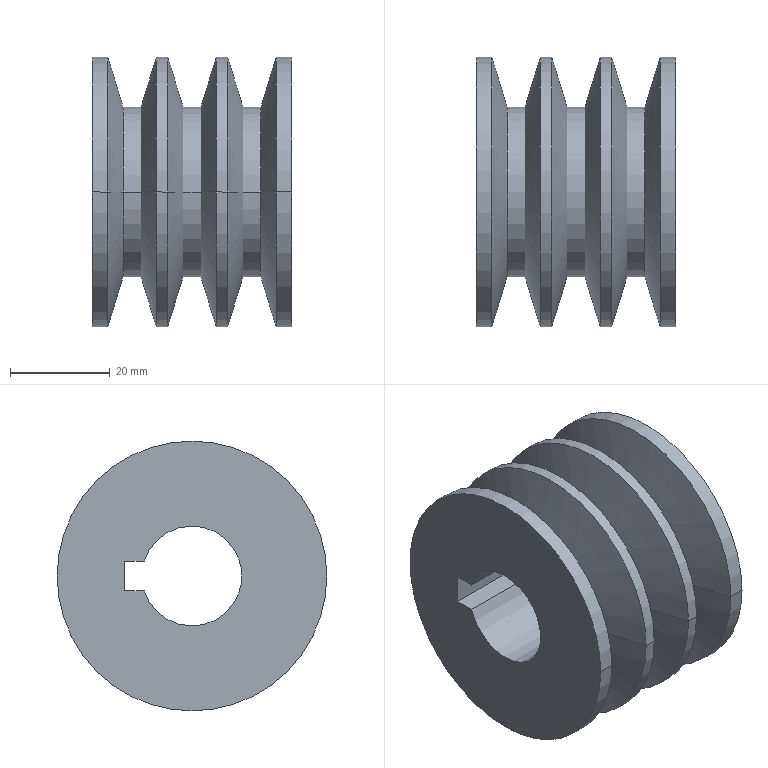Part | STEP file | Constant-speed small pulley | 1 solid | 32 faces | box 40 x 54 x 54 mm | volume 49564 mm3 | cylinder 15 | cone 12 | plane 5 | commonest cylinder face diameters 54 x8 34 x6 20 x1
STEP:
#1=CARTESIAN_POINT('',(-3.139,27.,0.));
#2=VERTEX_POINT('',#1);
#3=CARTESIAN_POINT('',(-3.139,-27.,0.));
#4=VERTEX_POINT('',#3);
#5=CARTESIAN_POINT('',(-3.139,0.,0.));
#6=DIRECTION('',(1.,0.,0.));
#7=DIRECTION('',(0.,1.,0.));
#8=AXIS2_PLACEMENT_3D('',#5,#6,#7);
#9=CIRCLE('',#8,27.);
#10=EDGE_CURVE('',#2,#4,#9,.T.);
#11=ORIENTED_EDGE('',*,*,#10,.T.);
#12=CARTESIAN_POINT('',(0.,-27.,0.));
#13=VERTEX_POINT('',#12);
#14=CARTESIAN_POINT('',(22.861,-27.,0.));
#15=DIRECTION('',(1.,0.,0.));
#16=VECTOR('',#15,1000.);
#17=LINE('',#14,#16);
#18=EDGE_CURVE('',#4,#13,#17,.T.);
#19=ORIENTED_EDGE('',*,*,#18,.T.);
#20=CARTESIAN_POINT('',(0.,27.,0.));
#21=VERTEX_POINT('',#20);
#22=CARTESIAN_POINT('',(0.,0.,0.));
#23=DIRECTION('',(1.,0.,0.));
#24=DIRECTION('',(0.,1.,0.));
#25=AXIS2_PLACEMENT_3D('',#22,#23,#24);
#26=CIRCLE('',#25,27.);
#27=EDGE_CURVE('',#21,#13,#26,.T.);
#28=ORIENTED_EDGE('',*,*,#27,.F.);
#29=CARTESIAN_POINT('',(22.861,27.,0.));
#30=DIRECTION('',(1.,0.,0.));
#31=VECTOR('',#30,1000.);
#32=LINE('',#29,#31);
#33=EDGE_CURVE('',#2,#21,#32,.T.);
#34=ORIENTED_EDGE('',*,*,#33,.F.);
#35=EDGE_LOOP('',(#11,#19,#28,#34));
#36=FACE_OUTER_BOUND('',#35,.T.);
#37=CARTESIAN_POINT('',(22.861,0.,0.));
#38=DIRECTION('',(1.,0.,0.));
#39=DIRECTION('',(0.,1.,0.));
#40=AXIS2_PLACEMENT_3D('',#37,#38,#39);
#41=CYLINDRICAL_SURFACE('',#40,27.);
#42=ADVANCED_FACE('',(#36),#41,.T.);
#43=CARTESIAN_POINT('',(3.057,17.,0.));
#44=VERTEX_POINT('',#43);
#45=CARTESIAN_POINT('',(3.057,-17.,0.));
#46=VERTEX_POINT('',#45);
#47=CARTESIAN_POINT('',(3.057,0.,0.));
#48=DIRECTION('',(1.,0.,0.));
#49=DIRECTION('',(0.,1.,0.));
#50=AXIS2_PLACEMENT_3D('',#47,#48,#49);
#51=CIRCLE('',#50,17.);
#52=EDGE_CURVE('',#44,#46,#51,.T.);
#53=ORIENTED_EDGE('',*,*,#52,.F.);
#54=CARTESIAN_POINT('',(3.057,17.,0.));
#55=DIRECTION('',(-0.2924,0.9563,0.));
#56=VECTOR('',#55,1000.);
#57=LINE('',#54,#56);
#58=EDGE_CURVE('',#44,#21,#57,.T.);
#59=ORIENTED_EDGE('',*,*,#58,.T.);
#60=ORIENTED_EDGE('',*,*,#27,.T.);
#61=CARTESIAN_POINT('',(3.057,-17.,0.));
#62=DIRECTION('',(-0.2924,-0.9563,0.));
#63=VECTOR('',#62,1000.);
#64=LINE('',#61,#63);
#65=EDGE_CURVE('',#46,#13,#64,.T.);
#66=ORIENTED_EDGE('',*,*,#65,.F.);
#67=EDGE_LOOP('',(#53,#59,#60,#66));
#68=FACE_OUTER_BOUND('',#67,.T.);
#69=CARTESIAN_POINT('',(3.057,0.,0.));
#70=DIRECTION('',(-1.,0.,0.));
#71=DIRECTION('',(0.,-1.,0.));
#72=AXIS2_PLACEMENT_3D('',#69,#70,#71);
#73=CONICAL_SURFACE('',#72,17.,1.274);
#74=ADVANCED_FACE('',(#68),#73,.T.);
#75=ORIENTED_EDGE('',*,*,#52,.T.);
#76=CARTESIAN_POINT('',(6.666,-17.,0.));
#77=VERTEX_POINT('',#76);
#78=CARTESIAN_POINT('',(22.861,-17.,0.));
#79=DIRECTION('',(1.,0.,0.));
#80=VECTOR('',#79,1000.);
#81=LINE('',#78,#80);
#82=EDGE_CURVE('',#46,#77,#81,.T.);
#83=ORIENTED_EDGE('',*,*,#82,.T.);
#84=CARTESIAN_POINT('',(6.666,17.,0.));
#85=VERTEX_POINT('',#84);
#86=CARTESIAN_POINT('',(6.666,0.,0.));
#87=DIRECTION('',(1.,0.,0.));
#88=DIRECTION('',(0.,1.,0.));
#89=AXIS2_PLACEMENT_3D('',#86,#87,#88);
#90=CIRCLE('',#89,17.);
#91=EDGE_CURVE('',#85,#77,#90,.T.);
#92=ORIENTED_EDGE('',*,*,#91,.F.);
#93=CARTESIAN_POINT('',(22.861,17.,0.));
#94=DIRECTION('',(1.,0.,0.));
#95=VECTOR('',#94,1000.);
#96=LINE('',#93,#95);
#97=EDGE_CURVE('',#44,#85,#96,.T.);
#98=ORIENTED_EDGE('',*,*,#97,.F.);
#99=EDGE_LOOP('',(#75,#83,#92,#98));
#100=FACE_OUTER_BOUND('',#99,.T.);
#101=CARTESIAN_POINT('',(22.861,0.,0.));
#102=DIRECTION('',(1.,0.,0.));
#103=DIRECTION('',(0.,1.,0.));
#104=AXIS2_PLACEMENT_3D('',#101,#102,#103);
#105=CYLINDRICAL_SURFACE('',#104,17.);
#106=ADVANCED_FACE('',(#100),#105,.T.);
#107=ORIENTED_EDGE('',*,*,#91,.T.);
#108=CARTESIAN_POINT('',(9.723,-27.,0.));
#109=VERTEX_POINT('',#108);
#110=CARTESIAN_POINT('',(9.723,-27.,0.));
#111=DIRECTION('',(0.2924,-0.9563,0.));
#112=VECTOR('',#111,1000.);
#113=LINE('',#110,#112);
#114=EDGE_CURVE('',#77,#109,#113,.T.);
#115=ORIENTED_EDGE('',*,*,#114,.T.);
#116=CARTESIAN_POINT('',(9.723,27.,0.));
#117=VERTEX_POINT('',#116);
#118=CARTESIAN_POINT('',(9.723,0.,0.));
#119=DIRECTION('',(1.,0.,0.));
#120=DIRECTION('',(0.,1.,0.));
#121=AXIS2_PLACEMENT_3D('',#118,#119,#120);
#122=CIRCLE('',#121,27.);
#123=EDGE_CURVE('',#117,#109,#122,.T.);
#124=ORIENTED_EDGE('',*,*,#123,.F.);
#125=CARTESIAN_POINT('',(9.723,27.,0.));
#126=DIRECTION('',(0.2924,0.9563,0.));
#127=VECTOR('',#126,1000.);
#128=LINE('',#125,#127);
#129=EDGE_CURVE('',#85,#117,#128,.T.);
#130=ORIENTED_EDGE('',*,*,#129,.F.);
#131=EDGE_LOOP('',(#107,#115,#124,#130));
#132=FACE_OUTER_BOUND('',#131,.T.);
#133=CARTESIAN_POINT('',(9.723,0.,0.));
#134=DIRECTION('',(1.,0.,0.));
#135=DIRECTION('',(0.,1.,0.));
#136=AXIS2_PLACEMENT_3D('',#133,#134,#135);
#137=CONICAL_SURFACE('',#136,27.,1.274);
#138=ADVANCED_FACE('',(#132),#137,.T.);
#139=ORIENTED_EDGE('',*,*,#123,.T.);
#140=CARTESIAN_POINT('',(12.,-27.,0.));
#141=VERTEX_POINT('',#140);
#142=CARTESIAN_POINT('',(22.861,-27.,0.));
#143=DIRECTION('',(1.,0.,0.));
#144=VECTOR('',#143,1000.);
#145=LINE('',#142,#144);
#146=EDGE_CURVE('',#109,#141,#145,.T.);
#147=ORIENTED_EDGE('',*,*,#146,.T.);
#148=CARTESIAN_POINT('',(12.,27.,0.));
#149=VERTEX_POINT('',#148);
#150=CARTESIAN_POINT('',(12.,0.,0.));
#151=DIRECTION('',(1.,0.,0.));
#152=DIRECTION('',(0.,1.,0.));
#153=AXIS2_PLACEMENT_3D('',#150,#151,#152);
#154=CIRCLE('',#153,27.);
#155=EDGE_CURVE('',#149,#141,#154,.T.);
#156=ORIENTED_EDGE('',*,*,#155,.F.);
#157=CARTESIAN_POINT('',(22.861,27.,0.));
#158=DIRECTION('',(1.,0.,0.));
#159=VECTOR('',#158,1000.);
#160=LINE('',#157,#159);
#161=EDGE_CURVE('',#117,#149,#160,.T.);
#162=ORIENTED_EDGE('',*,*,#161,.F.);
#163=EDGE_LOOP('',(#139,#147,#156,#162));
#164=FACE_OUTER_BOUND('',#163,.T.);
#165=CARTESIAN_POINT('',(22.861,0.,0.));
#166=DIRECTION('',(1.,0.,0.));
#167=DIRECTION('',(0.,1.,0.));
#168=AXIS2_PLACEMENT_3D('',#165,#166,#167);
#169=CYLINDRICAL_SURFACE('',#168,27.);
#170=ADVANCED_FACE('',(#164),#169,.T.);
#171=CARTESIAN_POINT('',(15.057,17.,0.));
#172=VERTEX_POINT('',#171);
#173=CARTESIAN_POINT('',(15.057,-17.,0.));
#174=VERTEX_POINT('',#173);
#175=CARTESIAN_POINT('',(15.057,0.,0.));
#176=DIRECTION('',(1.,0.,0.));
#177=DIRECTION('',(0.,1.,0.));
#178=AXIS2_PLACEMENT_3D('',#175,#176,#177);
#179=CIRCLE('',#178,17.);
#180=EDGE_CURVE('',#172,#174,#179,.T.);
#181=ORIENTED_EDGE('',*,*,#180,.F.);
#182=CARTESIAN_POINT('',(15.057,17.,0.));
#183=DIRECTION('',(-0.2924,0.9563,0.));
#184=VECTOR('',#183,1000.);
#185=LINE('',#182,#184);
#186=EDGE_CURVE('',#172,#149,#185,.T.);
#187=ORIENTED_EDGE('',*,*,#186,.T.);
#188=ORIENTED_EDGE('',*,*,#155,.T.);
#189=CARTESIAN_POINT('',(15.057,-17.,0.));
#190=DIRECTION('',(-0.2924,-0.9563,0.));
#191=VECTOR('',#190,1000.);
#192=LINE('',#189,#191);
#193=EDGE_CURVE('',#174,#141,#192,.T.);
#194=ORIENTED_EDGE('',*,*,#193,.F.);
#195=EDGE_LOOP('',(#181,#187,#188,#194));
#196=FACE_OUTER_BOUND('',#195,.T.);
#197=CARTESIAN_POINT('',(15.057,0.,0.));
#198=DIRECTION('',(-1.,0.,0.));
#199=DIRECTION('',(0.,-1.,0.));
#200=AXIS2_PLACEMENT_3D('',#197,#198,#199);
#201=CONICAL_SURFACE('',#200,17.,1.274);
#202=ADVANCED_FACE('',(#196),#201,.T.);
#203=ORIENTED_EDGE('',*,*,#180,.T.);
#204=CARTESIAN_POINT('',(18.666,-17.,0.));
#205=VERTEX_POINT('',#204);
#206=CARTESIAN_POINT('',(22.861,-17.,0.));
#207=DIRECTION('',(1.,0.,0.));
#208=VECTOR('',#207,1000.);
#209=LINE('',#206,#208);
#210=EDGE_CURVE('',#174,#205,#209,.T.);
#211=ORIENTED_EDGE('',*,*,#210,.T.);
#212=CARTESIAN_POINT('',(18.666,17.,0.));
#213=VERTEX_POINT('',#212);
#214=CARTESIAN_POINT('',(18.666,0.,0.));
#215=DIRECTION('',(1.,0.,0.));
#216=DIRECTION('',(0.,1.,0.));
#217=AXIS2_PLACEMENT_3D('',#214,#215,#216);
#218=CIRCLE('',#217,17.);
#219=EDGE_CURVE('',#213,#205,#218,.T.);
#220=ORIENTED_EDGE('',*,*,#219,.F.);
#221=CARTESIAN_POINT('',(22.861,17.,0.));
#222=DIRECTION('',(1.,0.,0.));
#223=VECTOR('',#222,1000.);
#224=LINE('',#221,#223);
#225=EDGE_CURVE('',#172,#213,#224,.T.);
#226=ORIENTED_EDGE('',*,*,#225,.F.);
#227=EDGE_LOOP('',(#203,#211,#220,#226));
#228=FACE_OUTER_BOUND('',#227,.T.);
#229=CARTESIAN_POINT('',(22.861,0.,0.));
#230=DIRECTION('',(1.,0.,0.));
#231=DIRECTION('',(0.,1.,0.));
#232=AXIS2_PLACEMENT_3D('',#229,#230,#231);
#233=CYLINDRICAL_SURFACE('',#232,17.);
#234=ADVANCED_FACE('',(#228),#233,.T.);
#235=ORIENTED_EDGE('',*,*,#219,.T.);
#236=CARTESIAN_POINT('',(21.723,-27.,0.));
#237=VERTEX_POINT('',#236);
#238=CARTESIAN_POINT('',(21.723,-27.,0.));
#239=DIRECTION('',(0.2924,-0.9563,0.));
#240=VECTOR('',#239,1000.);
#241=LINE('',#238,#240);
#242=EDGE_CURVE('',#205,#237,#241,.T.);
#243=ORIENTED_EDGE('',*,*,#242,.T.);
#244=CARTESIAN_POINT('',(21.723,27.,0.));
#245=VERTEX_POINT('',#244);
#246=CARTESIAN_POINT('',(21.723,0.,0.));
#247=DIRECTION('',(1.,0.,0.));
#248=DIRECTION('',(0.,1.,0.));
#249=AXIS2_PLACEMENT_3D('',#246,#247,#248);
#250=CIRCLE('',#249,27.);
#251=EDGE_CURVE('',#245,#237,#250,.T.);
#252=ORIENTED_EDGE('',*,*,#251,.F.);
#253=CARTESIAN_POINT('',(21.723,27.,0.));
#254=DIRECTION('',(0.2924,0.9563,0.));
#255=VECTOR('',#254,1000.);
#256=LINE('',#253,#255);
#257=EDGE_CURVE('',#213,#245,#256,.T.);
#258=ORIENTED_EDGE('',*,*,#257,.F.);
#259=EDGE_LOOP('',(#235,#243,#252,#258));
#260=FACE_OUTER_BOUND('',#259,.T.);
#261=CARTESIAN_POINT('',(21.723,0.,0.));
#262=DIRECTION('',(1.,0.,0.));
#263=DIRECTION('',(0.,1.,0.));
#264=AXIS2_PLACEMENT_3D('',#261,#262,#263);
#265=CONICAL_SURFACE('',#264,27.,1.274);
#266=ADVANCED_FACE('',(#260),#265,.T.);
#267=ORIENTED_EDGE('',*,*,#251,.T.);
#268=CARTESIAN_POINT('',(24.,-27.,0.));
#269=VERTEX_POINT('',#268);
#270=CARTESIAN_POINT('',(22.861,-27.,0.));
#271=DIRECTION('',(1.,0.,0.));
#272=VECTOR('',#271,1000.);
#273=LINE('',#270,#272);
#274=EDGE_CURVE('',#237,#269,#273,.T.);
#275=ORIENTED_EDGE('',*,*,#274,.T.);
#276=CARTESIAN_POINT('',(24.,27.,0.));
#277=VERTEX_POINT('',#276);
#278=CARTESIAN_POINT('',(24.,0.,0.));
#279=DIRECTION('',(1.,0.,0.));
#280=DIRECTION('',(0.,1.,0.));
#281=AXIS2_PLACEMENT_3D('',#278,#279,#280);
#282=CIRCLE('',#281,27.);
#283=EDGE_CURVE('',#277,#269,#282,.T.);
#284=ORIENTED_EDGE('',*,*,#283,.F.);
#285=CARTESIAN_POINT('',(22.861,27.,0.));
#286=DIRECTION('',(1.,0.,0.));
#287=VECTOR('',#286,1000.);
#288=LINE('',#285,#287);
#289=EDGE_CURVE('',#245,#277,#288,.T.);
#290=ORIENTED_EDGE('',*,*,#289,.F.);
#291=EDGE_LOOP('',(#267,#275,#284,#290));
#292=FACE_OUTER_BOUND('',#291,.T.);
#293=CARTESIAN_POINT('',(22.861,0.,0.));
#294=DIRECTION('',(1.,0.,0.));
#295=DIRECTION('',(0.,1.,0.));
#296=AXIS2_PLACEMENT_3D('',#293,#294,#295);
#297=CYLINDRICAL_SURFACE('',#296,27.);
#298=ADVANCED_FACE('',(#292),#297,.T.);
#299=CARTESIAN_POINT('',(27.057,17.,0.));
#300=VERTEX_POINT('',#299);
#301=CARTESIAN_POINT('',(27.057,-17.,0.));
#302=VERTEX_POINT('',#301);
#303=CARTESIAN_POINT('',(27.057,0.,0.));
#304=DIRECTION('',(1.,0.,0.));
#305=DIRECTION('',(0.,1.,0.));
#306=AXIS2_PLACEMENT_3D('',#303,#304,#305);
#307=CIRCLE('',#306,17.);
#308=EDGE_CURVE('',#300,#302,#307,.T.);
#309=ORIENTED_EDGE('',*,*,#308,.F.);
#310=CARTESIAN_POINT('',(27.057,17.,0.));
#311=DIRECTION('',(-0.2924,0.9563,0.));
#312=VECTOR('',#311,1000.);
#313=LINE('',#310,#312);
#314=EDGE_CURVE('',#300,#277,#313,.T.);
#315=ORIENTED_EDGE('',*,*,#314,.T.);
#316=ORIENTED_EDGE('',*,*,#283,.T.);
#317=CARTESIAN_POINT('',(27.057,-17.,0.));
#318=DIRECTION('',(-0.2924,-0.9563,0.));
#319=VECTOR('',#318,1000.);
#320=LINE('',#317,#319);
#321=EDGE_CURVE('',#302,#269,#320,.T.);
#322=ORIENTED_EDGE('',*,*,#321,.F.);
#323=EDGE_LOOP('',(#309,#315,#316,#322));
#324=FACE_OUTER_BOUND('',#323,.T.);
#325=CARTESIAN_POINT('',(27.057,0.,0.));
#326=DIRECTION('',(-1.,0.,0.));
#327=DIRECTION('',(0.,-1.,0.));
#328=AXIS2_PLACEMENT_3D('',#325,#326,#327);
#329=CONICAL_SURFACE('',#328,17.,1.274);
#330=ADVANCED_FACE('',(#324),#329,.T.);
#331=ORIENTED_EDGE('',*,*,#308,.T.);
#332=CARTESIAN_POINT('',(30.666,-17.,0.));
#333=VERTEX_POINT('',#332);
#334=CARTESIAN_POINT('',(22.861,-17.,0.));
#335=DIRECTION('',(1.,0.,0.));
#336=VECTOR('',#335,1000.);
#337=LINE('',#334,#336);
#338=EDGE_CURVE('',#302,#333,#337,.T.);
#339=ORIENTED_EDGE('',*,*,#338,.T.);
#340=CARTESIAN_POINT('',(30.666,17.,0.));
#341=VERTEX_POINT('',#340);
#342=CARTESIAN_POINT('',(30.666,0.,0.));
#343=DIRECTION('',(1.,0.,0.));
#344=DIRECTION('',(0.,1.,0.));
#345=AXIS2_PLACEMENT_3D('',#342,#343,#344);
#346=CIRCLE('',#345,17.);
#347=EDGE_CURVE('',#341,#333,#346,.T.);
#348=ORIENTED_EDGE('',*,*,#347,.F.);
#349=CARTESIAN_POINT('',(22.861,17.,0.));
#350=DIRECTION('',(1.,0.,0.));
#351=VECTOR('',#350,1000.);
#352=LINE('',#349,#351);
#353=EDGE_CURVE('',#300,#341,#352,.T.);
#354=ORIENTED_EDGE('',*,*,#353,.F.);
#355=EDGE_LOOP('',(#331,#339,#348,#354));
#356=FACE_OUTER_BOUND('',#355,.T.);
#357=CARTESIAN_POINT('',(22.861,0.,0.));
#358=DIRECTION('',(1.,0.,0.));
#359=DIRECTION('',(0.,1.,0.));
#360=AXIS2_PLACEMENT_3D('',#357,#358,#359);
#361=CYLINDRICAL_SURFACE('',#360,17.);
#362=ADVANCED_FACE('',(#356),#361,.T.);
#363=ORIENTED_EDGE('',*,*,#347,.T.);
#364=CARTESIAN_POINT('',(33.723,-27.,0.));
#365=VERTEX_POINT('',#364);
#366=CARTESIAN_POINT('',(33.723,-27.,0.));
#367=DIRECTION('',(0.2924,-0.9563,0.));
#368=VECTOR('',#367,1000.);
#369=LINE('',#366,#368);
#370=EDGE_CURVE('',#333,#365,#369,.T.);
#371=ORIENTED_EDGE('',*,*,#370,.T.);
#372=CARTESIAN_POINT('',(33.723,27.,0.));
#373=VERTEX_POINT('',#372);
#374=CARTESIAN_POINT('',(33.723,0.,0.));
#375=DIRECTION('',(1.,0.,0.));
#376=DIRECTION('',(0.,1.,0.));
#377=AXIS2_PLACEMENT_3D('',#374,#375,#376);
#378=CIRCLE('',#377,27.);
#379=EDGE_CURVE('',#373,#365,#378,.T.);
#380=ORIENTED_EDGE('',*,*,#379,.F.);
#381=CARTESIAN_POINT('',(33.723,27.,0.));
#382=DIRECTION('',(0.2924,0.9563,0.));
#383=VECTOR('',#382,1000.);
#384=LINE('',#381,#383);
#385=EDGE_CURVE('',#341,#373,#384,.T.);
#386=ORIENTED_EDGE('',*,*,#385,.F.);
#387=EDGE_LOOP('',(#363,#371,#380,#386));
#388=FACE_OUTER_BOUND('',#387,.T.);
#389=CARTESIAN_POINT('',(33.723,0.,0.));
#390=DIRECTION('',(1.,0.,0.));
#391=DIRECTION('',(0.,1.,0.));
#392=AXIS2_PLACEMENT_3D('',#389,#390,#391);
#393=CONICAL_SURFACE('',#392,27.,1.274);
#394=ADVANCED_FACE('',(#388),#393,.T.);
#395=ORIENTED_EDGE('',*,*,#379,.T.);
#396=CARTESIAN_POINT('',(36.861,-27.,0.));
#397=VERTEX_POINT('',#396);
#398=CARTESIAN_POINT('',(22.861,-27.,0.));
#399=DIRECTION('',(1.,0.,0.));
#400=VECTOR('',#399,1000.);
#401=LINE('',#398,#400);
#402=EDGE_CURVE('',#365,#397,#401,.T.);
#403=ORIENTED_EDGE('',*,*,#402,.T.);
#404=CARTESIAN_POINT('',(36.861,27.,0.));
#405=VERTEX_POINT('',#404);
#406=CARTESIAN_POINT('',(36.861,0.,0.));
#407=DIRECTION('',(1.,0.,0.));
#408=DIRECTION('',(0.,1.,0.));
#409=AXIS2_PLACEMENT_3D('',#406,#407,#408);
#410=CIRCLE('',#409,27.);
#411=EDGE_CURVE('',#405,#397,#410,.T.);
#412=ORIENTED_EDGE('',*,*,#411,.F.);
#413=CARTESIAN_POINT('',(22.861,27.,0.));
#414=DIRECTION('',(1.,0.,0.));
#415=VECTOR('',#414,1000.);
#416=LINE('',#413,#415);
#417=EDGE_CURVE('',#373,#405,#416,.T.);
#418=ORIENTED_EDGE('',*,*,#417,.F.);
#419=EDGE_LOOP('',(#395,#403,#412,#418));
#420=FACE_OUTER_BOUND('',#419,.T.);
#421=CARTESIAN_POINT('',(22.861,0.,0.));
#422=DIRECTION('',(1.,0.,0.));
#423=DIRECTION('',(0.,1.,0.));
#424=AXIS2_PLACEMENT_3D('',#421,#422,#423);
#425=CYLINDRICAL_SURFACE('',#424,27.);
#426=ADVANCED_FACE('',(#420),#425,.T.);
#427=CARTESIAN_POINT('',(-3.139,13.5,-3.));
#428=VERTEX_POINT('',#427);
#429=CARTESIAN_POINT('',(-3.139,9.539,-3.));
#430=VERTEX_POINT('',#429);
#431=CARTESIAN_POINT('',(-3.139,27.,-3.));
#432=DIRECTION('',(0.,-1.,0.));
#433=VECTOR('',#432,1000.);
#434=LINE('',#431,#433);
#435=EDGE_CURVE('',#428,#430,#434,.T.);
#436=ORIENTED_EDGE('',*,*,#435,.F.);
#437=CARTESIAN_POINT('',(-3.139,13.5,3.));
#438=VERTEX_POINT('',#437);
#439=CARTESIAN_POINT('',(-3.139,13.5,0.));
#440=DIRECTION('',(0.,0.,-1.));
#441=VECTOR('',#440,1000.);
#442=LINE('',#439,#441);
#443=EDGE_CURVE('',#438,#428,#442,.T.);
#444=ORIENTED_EDGE('',*,*,#443,.F.);
#445=CARTESIAN_POINT('',(-3.139,9.539,3.));
#446=VERTEX_POINT('',#445);
#447=CARTESIAN_POINT('',(-3.139,27.,3.));
#448=DIRECTION('',(0.,1.,0.));
#449=VECTOR('',#448,1000.);
#450=LINE('',#447,#449);
#451=EDGE_CURVE('',#446,#438,#450,.T.);
#452=ORIENTED_EDGE('',*,*,#451,.F.);
#453=CARTESIAN_POINT('',(-3.139,0.,0.));
#454=DIRECTION('',(-1.,0.,0.));
#455=DIRECTION('',(0.,-1.,0.));
#456=AXIS2_PLACEMENT_3D('',#453,#454,#455);
#457=CIRCLE('',#456,10.);
#458=EDGE_CURVE('',#430,#446,#457,.T.);
#459=ORIENTED_EDGE('',*,*,#458,.F.);
#460=EDGE_LOOP('',(#436,#444,#452,#459));
#461=FACE_BOUND('',#460,.T.);
#462=ORIENTED_EDGE('',*,*,#10,.F.);
#463=CARTESIAN_POINT('',(-3.139,0.,0.));
#464=DIRECTION('',(1.,0.,0.));
#465=DIRECTION('',(0.,1.,0.));
#466=AXIS2_PLACEMENT_3D('',#463,#464,#465);
#467=CIRCLE('',#466,27.);
#468=EDGE_CURVE('',#4,#2,#467,.T.);
#469=ORIENTED_EDGE('',*,*,#468,.F.);
#470=EDGE_LOOP('',(#462,#469));
#471=FACE_OUTER_BOUND('',#470,.T.);
#472=CARTESIAN_POINT('',(-3.139,27.,0.));
#473=DIRECTION('',(-1.,0.,0.));
#474=DIRECTION('',(0.,-1.,0.));
#475=AXIS2_PLACEMENT_3D('',#472,#473,#474);
#476=PLANE('',#475);
#477=ADVANCED_FACE('',(#461,#471),#476,.T.);
#478=CARTESIAN_POINT('',(36.861,9.539,-3.));
#479=VERTEX_POINT('',#478);
#480=CARTESIAN_POINT('',(36.861,13.5,-3.));
#481=VERTEX_POINT('',#480);
#482=CARTESIAN_POINT('',(36.861,13.5,-3.));
#483=DIRECTION('',(0.,1.,0.));
#484=VECTOR('',#483,1000.);
#485=LINE('',#482,#484);
#486=EDGE_CURVE('',#479,#481,#485,.T.);
#487=ORIENTED_EDGE('',*,*,#486,.F.);
#488=CARTESIAN_POINT('',(36.861,9.539,3.));
#489=VERTEX_POINT('',#488);
#490=CARTESIAN_POINT('',(36.861,0.,0.));
#491=DIRECTION('',(1.,0.,0.));
#492=DIRECTION('',(0.,1.,0.));
#493=AXIS2_PLACEMENT_3D('',#490,#491,#492);
#494=CIRCLE('',#493,10.);
#495=EDGE_CURVE('',#489,#479,#494,.T.);
#496=ORIENTED_EDGE('',*,*,#495,.F.);
#497=CARTESIAN_POINT('',(36.861,13.5,3.));
#498=VERTEX_POINT('',#497);
#499=CARTESIAN_POINT('',(36.861,13.5,3.));
#500=DIRECTION('',(0.,-1.,0.));
#501=VECTOR('',#500,1000.);
#502=LINE('',#499,#501);
#503=EDGE_CURVE('',#498,#489,#502,.T.);
#504=ORIENTED_EDGE('',*,*,#503,.F.);
#505=CARTESIAN_POINT('',(36.861,13.5,3.));
#506=DIRECTION('',(0.,0.,1.));
#507=VECTOR('',#506,1000.);
#508=LINE('',#505,#507);
#509=EDGE_CURVE('',#481,#498,#508,.T.);
#510=ORIENTED_EDGE('',*,*,#509,.F.);
#511=EDGE_LOOP('',(#487,#496,#504,#510));
#512=FACE_BOUND('',#511,.T.);
#513=ORIENTED_EDGE('',*,*,#411,.T.);
#514=CARTESIAN_POINT('',(36.861,0.,0.));
#515=DIRECTION('',(1.,0.,0.));
#516=DIRECTION('',(0.,1.,0.));
#517=AXIS2_PLACEMENT_3D('',#514,#515,#516);
#518=CIRCLE('',#517,27.);
#519=EDGE_CURVE('',#397,#405,#518,.T.);
#520=ORIENTED_EDGE('',*,*,#519,.T.);
#521=EDGE_LOOP('',(#513,#520));
#522=FACE_OUTER_BOUND('',#521,.T.);
#523=CARTESIAN_POINT('',(36.861,27.,0.));
#524=DIRECTION('',(1.,0.,0.));
#525=DIRECTION('',(0.,1.,0.));
#526=AXIS2_PLACEMENT_3D('',#523,#524,#525);
#527=PLANE('',#526);
#528=ADVANCED_FACE('',(#512,#522),#527,.T.);
#529=ORIENTED_EDGE('',*,*,#402,.F.);
#530=CARTESIAN_POINT('',(33.723,0.,0.));
#531=DIRECTION('',(1.,0.,0.));
#532=DIRECTION('',(0.,1.,0.));
#533=AXIS2_PLACEMENT_3D('',#530,#531,#532);
#534=CIRCLE('',#533,27.);
#535=EDGE_CURVE('',#365,#373,#534,.T.);
#536=ORIENTED_EDGE('',*,*,#535,.T.);
#537=ORIENTED_EDGE('',*,*,#417,.T.);
#538=ORIENTED_EDGE('',*,*,#519,.F.);
#539=EDGE_LOOP('',(#529,#536,#537,#538));
#540=FACE_OUTER_BOUND('',#539,.T.);
#541=CARTESIAN_POINT('',(22.861,0.,0.));
#542=DIRECTION('',(1.,0.,0.));
#543=DIRECTION('',(0.,1.,0.));
#544=AXIS2_PLACEMENT_3D('',#541,#542,#543);
#545=CYLINDRICAL_SURFACE('',#544,27.);
#546=ADVANCED_FACE('',(#540),#545,.T.);
#547=ORIENTED_EDGE('',*,*,#370,.F.);
#548=CARTESIAN_POINT('',(30.666,0.,0.));
#549=DIRECTION('',(1.,0.,0.));
#550=DIRECTION('',(0.,1.,0.));
#551=AXIS2_PLACEMENT_3D('',#548,#549,#550);
#552=CIRCLE('',#551,17.);
#553=EDGE_CURVE('',#333,#341,#552,.T.);
#554=ORIENTED_EDGE('',*,*,#553,.T.);
#555=ORIENTED_EDGE('',*,*,#385,.T.);
#556=ORIENTED_EDGE('',*,*,#535,.F.);
#557=EDGE_LOOP('',(#547,#554,#555,#556));
#558=FACE_OUTER_BOUND('',#557,.T.);
#559=CARTESIAN_POINT('',(33.723,0.,0.));
#560=DIRECTION('',(1.,0.,0.));
#561=DIRECTION('',(0.,1.,0.));
#562=AXIS2_PLACEMENT_3D('',#559,#560,#561);
#563=CONICAL_SURFACE('',#562,27.,1.274);
#564=ADVANCED_FACE('',(#558),#563,.T.);
#565=ORIENTED_EDGE('',*,*,#338,.F.);
#566=CARTESIAN_POINT('',(27.057,0.,0.));
#567=DIRECTION('',(1.,0.,0.));
#568=DIRECTION('',(0.,1.,0.));
#569=AXIS2_PLACEMENT_3D('',#566,#567,#568);
#570=CIRCLE('',#569,17.);
#571=EDGE_CURVE('',#302,#300,#570,.T.);
#572=ORIENTED_EDGE('',*,*,#571,.T.);
#573=ORIENTED_EDGE('',*,*,#353,.T.);
#574=ORIENTED_EDGE('',*,*,#553,.F.);
#575=EDGE_LOOP('',(#565,#572,#573,#574));
#576=FACE_OUTER_BOUND('',#575,.T.);
#577=CARTESIAN_POINT('',(22.861,0.,0.));
#578=DIRECTION('',(1.,0.,0.));
#579=DIRECTION('',(0.,1.,0.));
#580=AXIS2_PLACEMENT_3D('',#577,#578,#579);
#581=CYLINDRICAL_SURFACE('',#580,17.);
#582=ADVANCED_FACE('',(#576),#581,.T.);
#583=ORIENTED_EDGE('',*,*,#314,.F.);
#584=ORIENTED_EDGE('',*,*,#571,.F.);
#585=ORIENTED_EDGE('',*,*,#321,.T.);
#586=CARTESIAN_POINT('',(24.,0.,0.));
#587=DIRECTION('',(1.,0.,0.));
#588=DIRECTION('',(0.,1.,0.));
#589=AXIS2_PLACEMENT_3D('',#586,#587,#588);
#590=CIRCLE('',#589,27.);
#591=EDGE_CURVE('',#269,#277,#590,.T.);
#592=ORIENTED_EDGE('',*,*,#591,.T.);
#593=EDGE_LOOP('',(#583,#584,#585,#592));
#594=FACE_OUTER_BOUND('',#593,.T.);
#595=CARTESIAN_POINT('',(27.057,0.,0.));
#596=DIRECTION('',(-1.,0.,0.));
#597=DIRECTION('',(0.,-1.,0.));
#598=AXIS2_PLACEMENT_3D('',#595,#596,#597);
#599=CONICAL_SURFACE('',#598,17.,1.274);
#600=ADVANCED_FACE('',(#594),#599,.T.);
#601=ORIENTED_EDGE('',*,*,#274,.F.);
#602=CARTESIAN_POINT('',(21.723,0.,0.));
#603=DIRECTION('',(1.,0.,0.));
#604=DIRECTION('',(0.,1.,0.));
#605=AXIS2_PLACEMENT_3D('',#602,#603,#604);
#606=CIRCLE('',#605,27.);
#607=EDGE_CURVE('',#237,#245,#606,.T.);
#608=ORIENTED_EDGE('',*,*,#607,.T.);
#609=ORIENTED_EDGE('',*,*,#289,.T.);
#610=ORIENTED_EDGE('',*,*,#591,.F.);
#611=EDGE_LOOP('',(#601,#608,#609,#610));
#612=FACE_OUTER_BOUND('',#611,.T.);
#613=CARTESIAN_POINT('',(22.861,0.,0.));
#614=DIRECTION('',(1.,0.,0.));
#615=DIRECTION('',(0.,1.,0.));
#616=AXIS2_PLACEMENT_3D('',#613,#614,#615);
#617=CYLINDRICAL_SURFACE('',#616,27.);
#618=ADVANCED_FACE('',(#612),#617,.T.);
#619=ORIENTED_EDGE('',*,*,#242,.F.);
#620=CARTESIAN_POINT('',(18.666,0.,0.));
#621=DIRECTION('',(1.,0.,0.));
#622=DIRECTION('',(0.,1.,0.));
#623=AXIS2_PLACEMENT_3D('',#620,#621,#622);
#624=CIRCLE('',#623,17.);
#625=EDGE_CURVE('',#205,#213,#624,.T.);
#626=ORIENTED_EDGE('',*,*,#625,.T.);
#627=ORIENTED_EDGE('',*,*,#257,.T.);
#628=ORIENTED_EDGE('',*,*,#607,.F.);
#629=EDGE_LOOP('',(#619,#626,#627,#628));
#630=FACE_OUTER_BOUND('',#629,.T.);
#631=CARTESIAN_POINT('',(21.723,0.,0.));
#632=DIRECTION('',(1.,0.,0.));
#633=DIRECTION('',(0.,1.,0.));
#634=AXIS2_PLACEMENT_3D('',#631,#632,#633);
#635=CONICAL_SURFACE('',#634,27.,1.274);
#636=ADVANCED_FACE('',(#630),#635,.T.);
#637=ORIENTED_EDGE('',*,*,#210,.F.);
#638=CARTESIAN_POINT('',(15.057,0.,0.));
#639=DIRECTION('',(1.,0.,0.));
#640=DIRECTION('',(0.,1.,0.));
#641=AXIS2_PLACEMENT_3D('',#638,#639,#640);
#642=CIRCLE('',#641,17.);
#643=EDGE_CURVE('',#174,#172,#642,.T.);
#644=ORIENTED_EDGE('',*,*,#643,.T.);
#645=ORIENTED_EDGE('',*,*,#225,.T.);
#646=ORIENTED_EDGE('',*,*,#625,.F.);
#647=EDGE_LOOP('',(#637,#644,#645,#646));
#648=FACE_OUTER_BOUND('',#647,.T.);
#649=CARTESIAN_POINT('',(22.861,0.,0.));
#650=DIRECTION('',(1.,0.,0.));
#651=DIRECTION('',(0.,1.,0.));
#652=AXIS2_PLACEMENT_3D('',#649,#650,#651);
#653=CYLINDRICAL_SURFACE('',#652,17.);
#654=ADVANCED_FACE('',(#648),#653,.T.);
#655=ORIENTED_EDGE('',*,*,#186,.F.);
#656=ORIENTED_EDGE('',*,*,#643,.F.);
#657=ORIENTED_EDGE('',*,*,#193,.T.);
#658=CARTESIAN_POINT('',(12.,0.,0.));
#659=DIRECTION('',(1.,0.,0.));
#660=DIRECTION('',(0.,1.,0.));
#661=AXIS2_PLACEMENT_3D('',#658,#659,#660);
#662=CIRCLE('',#661,27.);
#663=EDGE_CURVE('',#141,#149,#662,.T.);
#664=ORIENTED_EDGE('',*,*,#663,.T.);
#665=EDGE_LOOP('',(#655,#656,#657,#664));
#666=FACE_OUTER_BOUND('',#665,.T.);
#667=CARTESIAN_POINT('',(15.057,0.,0.));
#668=DIRECTION('',(-1.,0.,0.));
#669=DIRECTION('',(0.,-1.,0.));
#670=AXIS2_PLACEMENT_3D('',#667,#668,#669);
#671=CONICAL_SURFACE('',#670,17.,1.274);
#672=ADVANCED_FACE('',(#666),#671,.T.);
#673=ORIENTED_EDGE('',*,*,#146,.F.);
#674=CARTESIAN_POINT('',(9.723,0.,0.));
#675=DIRECTION('',(1.,0.,0.));
#676=DIRECTION('',(0.,1.,0.));
#677=AXIS2_PLACEMENT_3D('',#674,#675,#676);
#678=CIRCLE('',#677,27.);
#679=EDGE_CURVE('',#109,#117,#678,.T.);
#680=ORIENTED_EDGE('',*,*,#679,.T.);
#681=ORIENTED_EDGE('',*,*,#161,.T.);
#682=ORIENTED_EDGE('',*,*,#663,.F.);
#683=EDGE_LOOP('',(#673,#680,#681,#682));
#684=FACE_OUTER_BOUND('',#683,.T.);
#685=CARTESIAN_POINT('',(22.861,0.,0.));
#686=DIRECTION('',(1.,0.,0.));
#687=DIRECTION('',(0.,1.,0.));
#688=AXIS2_PLACEMENT_3D('',#685,#686,#687);
#689=CYLINDRICAL_SURFACE('',#688,27.);
#690=ADVANCED_FACE('',(#684),#689,.T.);
#691=ORIENTED_EDGE('',*,*,#114,.F.);
#692=CARTESIAN_POINT('',(6.666,0.,0.));
#693=DIRECTION('',(1.,0.,0.));
#694=DIRECTION('',(0.,1.,0.));
#695=AXIS2_PLACEMENT_3D('',#692,#693,#694);
#696=CIRCLE('',#695,17.);
#697=EDGE_CURVE('',#77,#85,#696,.T.);
#698=ORIENTED_EDGE('',*,*,#697,.T.);
#699=ORIENTED_EDGE('',*,*,#129,.T.);
#700=ORIENTED_EDGE('',*,*,#679,.F.);
#701=EDGE_LOOP('',(#691,#698,#699,#700));
#702=FACE_OUTER_BOUND('',#701,.T.);
#703=CARTESIAN_POINT('',(9.723,0.,0.));
#704=DIRECTION('',(1.,0.,0.));
#705=DIRECTION('',(0.,1.,0.));
#706=AXIS2_PLACEMENT_3D('',#703,#704,#705);
#707=CONICAL_SURFACE('',#706,27.,1.274);
#708=ADVANCED_FACE('',(#702),#707,.T.);
#709=ORIENTED_EDGE('',*,*,#82,.F.);
#710=CARTESIAN_POINT('',(3.057,0.,0.));
#711=DIRECTION('',(1.,0.,0.));
#712=DIRECTION('',(0.,1.,0.));
#713=AXIS2_PLACEMENT_3D('',#710,#711,#712);
#714=CIRCLE('',#713,17.);
#715=EDGE_CURVE('',#46,#44,#714,.T.);
#716=ORIENTED_EDGE('',*,*,#715,.T.);
#717=ORIENTED_EDGE('',*,*,#97,.T.);
#718=ORIENTED_EDGE('',*,*,#697,.F.);
#719=EDGE_LOOP('',(#709,#716,#717,#718));
#720=FACE_OUTER_BOUND('',#719,.T.);
#721=CARTESIAN_POINT('',(22.861,0.,0.));
#722=DIRECTION('',(1.,0.,0.));
#723=DIRECTION('',(0.,1.,0.));
#724=AXIS2_PLACEMENT_3D('',#721,#722,#723);
#725=CYLINDRICAL_SURFACE('',#724,17.);
#726=ADVANCED_FACE('',(#720),#725,.T.);
#727=ORIENTED_EDGE('',*,*,#58,.F.);
#728=ORIENTED_EDGE('',*,*,#715,.F.);
#729=ORIENTED_EDGE('',*,*,#65,.T.);
#730=CARTESIAN_POINT('',(0.,0.,0.));
#731=DIRECTION('',(1.,0.,0.));
#732=DIRECTION('',(0.,1.,0.));
#733=AXIS2_PLACEMENT_3D('',#730,#731,#732);
#734=CIRCLE('',#733,27.);
#735=EDGE_CURVE('',#13,#21,#734,.T.);
#736=ORIENTED_EDGE('',*,*,#735,.T.);
#737=EDGE_LOOP('',(#727,#728,#729,#736));
#738=FACE_OUTER_BOUND('',#737,.T.);
#739=CARTESIAN_POINT('',(3.057,0.,0.));
#740=DIRECTION('',(-1.,0.,0.));
#741=DIRECTION('',(0.,-1.,0.));
#742=AXIS2_PLACEMENT_3D('',#739,#740,#741);
#743=CONICAL_SURFACE('',#742,17.,1.274);
#744=ADVANCED_FACE('',(#738),#743,.T.);
#745=ORIENTED_EDGE('',*,*,#18,.F.);
#746=ORIENTED_EDGE('',*,*,#468,.T.);
#747=ORIENTED_EDGE('',*,*,#33,.T.);
#748=ORIENTED_EDGE('',*,*,#735,.F.);
#749=EDGE_LOOP('',(#745,#746,#747,#748));
#750=FACE_OUTER_BOUND('',#749,.T.);
#751=CARTESIAN_POINT('',(22.861,0.,0.));
#752=DIRECTION('',(1.,0.,0.));
#753=DIRECTION('',(0.,1.,0.));
#754=AXIS2_PLACEMENT_3D('',#751,#752,#753);
#755=CYLINDRICAL_SURFACE('',#754,27.);
#756=ADVANCED_FACE('',(#750),#755,.T.);
#757=ORIENTED_EDGE('',*,*,#495,.T.);
#758=CARTESIAN_POINT('',(-19.139,9.539,-3.));
#759=DIRECTION('',(-1.,0.,0.));
#760=VECTOR('',#759,1000.);
#761=LINE('',#758,#760);
#762=EDGE_CURVE('',#479,#430,#761,.T.);
#763=ORIENTED_EDGE('',*,*,#762,.T.);
#764=ORIENTED_EDGE('',*,*,#458,.T.);
#765=CARTESIAN_POINT('',(-19.139,9.539,3.));
#766=DIRECTION('',(1.,0.,0.));
#767=VECTOR('',#766,1000.);
#768=LINE('',#765,#767);
#769=EDGE_CURVE('',#446,#489,#768,.T.);
#770=ORIENTED_EDGE('',*,*,#769,.T.);
#771=EDGE_LOOP('',(#757,#763,#764,#770));
#772=FACE_OUTER_BOUND('',#771,.T.);
#773=CARTESIAN_POINT('',(-19.139,0.,0.));
#774=DIRECTION('',(1.,0.,0.));
#775=DIRECTION('',(0.,1.,0.));
#776=AXIS2_PLACEMENT_3D('',#773,#774,#775);
#777=CYLINDRICAL_SURFACE('',#776,10.);
#778=ADVANCED_FACE('',(#772),#777,.F.);
#779=ORIENTED_EDGE('',*,*,#435,.T.);
#780=ORIENTED_EDGE('',*,*,#762,.F.);
#781=ORIENTED_EDGE('',*,*,#486,.T.);
#782=CARTESIAN_POINT('',(-19.139,13.5,-3.));
#783=DIRECTION('',(1.,0.,0.));
#784=VECTOR('',#783,1000.);
#785=LINE('',#782,#784);
#786=EDGE_CURVE('',#428,#481,#785,.T.);
#787=ORIENTED_EDGE('',*,*,#786,.F.);
#788=EDGE_LOOP('',(#779,#780,#781,#787));
#789=FACE_OUTER_BOUND('',#788,.T.);
#790=CARTESIAN_POINT('',(-19.139,13.5,-3.));
#791=DIRECTION('',(0.,0.,-1.));
#792=DIRECTION('',(-1.,0.,0.));
#793=AXIS2_PLACEMENT_3D('',#790,#791,#792);
#794=PLANE('',#793);
#795=ADVANCED_FACE('',(#789),#794,.F.);
#796=ORIENTED_EDGE('',*,*,#451,.T.);
#797=CARTESIAN_POINT('',(-19.139,13.5,3.));
#798=DIRECTION('',(1.,0.,0.));
#799=VECTOR('',#798,1000.);
#800=LINE('',#797,#799);
#801=EDGE_CURVE('',#438,#498,#800,.T.);
#802=ORIENTED_EDGE('',*,*,#801,.T.);
#803=ORIENTED_EDGE('',*,*,#503,.T.);
#804=ORIENTED_EDGE('',*,*,#769,.F.);
#805=EDGE_LOOP('',(#796,#802,#803,#804));
#806=FACE_OUTER_BOUND('',#805,.T.);
#807=CARTESIAN_POINT('',(-19.139,13.5,3.));
#808=DIRECTION('',(0.,0.,1.));
#809=DIRECTION('',(1.,0.,0.));
#810=AXIS2_PLACEMENT_3D('',#807,#808,#809);
#811=PLANE('',#810);
#812=ADVANCED_FACE('',(#806),#811,.F.);
#813=ORIENTED_EDGE('',*,*,#443,.T.);
#814=ORIENTED_EDGE('',*,*,#786,.T.);
#815=ORIENTED_EDGE('',*,*,#509,.T.);
#816=ORIENTED_EDGE('',*,*,#801,.F.);
#817=EDGE_LOOP('',(#813,#814,#815,#816));
#818=FACE_OUTER_BOUND('',#817,.T.);
#819=CARTESIAN_POINT('',(-19.139,13.5,3.));
#820=DIRECTION('',(0.,1.,0.));
#821=DIRECTION('',(-1.,0.,0.));
#822=AXIS2_PLACEMENT_3D('',#819,#820,#821);
#823=PLANE('',#822);
#824=ADVANCED_FACE('',(#818),#823,.F.);
#825=CLOSED_SHELL('',(#42,#74,#106,#138,#170,#202,#234,#266,#298,#330,#362,#394,#426,#477,#528,#546,#564,#582,#600,#618,#636,#654,#672,#690,#708,#726,#744,#756,#778,#795,#812,#824));
#826=MANIFOLD_SOLID_BREP('',#825);
#827=CARTESIAN_POINT('',(0.,0.,0.));
#828=DIRECTION('',(0.,0.,1.));
#829=DIRECTION('',(1.,0.,0.));
#830=AXIS2_PLACEMENT_3D('',#827,#828,#829);
#831=(LENGTH_UNIT()NAMED_UNIT(*)SI_UNIT(.MILLI.,.METRE.));
#832=UNCERTAINTY_MEASURE_WITH_UNIT(LENGTH_MEASURE(0.00001),#831,'','');
#833=(NAMED_UNIT(*)PLANE_ANGLE_UNIT()SI_UNIT($,.RADIAN.));
#834=(NAMED_UNIT(*)SI_UNIT($,.STERADIAN.)SOLID_ANGLE_UNIT());
#835=(GEOMETRIC_REPRESENTATION_CONTEXT(3)GLOBAL_UNCERTAINTY_ASSIGNED_CONTEXT((#832))GLOBAL_UNIT_ASSIGNED_CONTEXT((#831,#833,#834))REPRESENTATION_CONTEXT('',''));
#836=ADVANCED_BREP_SHAPE_REPRESENTATION('',(#826,#830),#835);